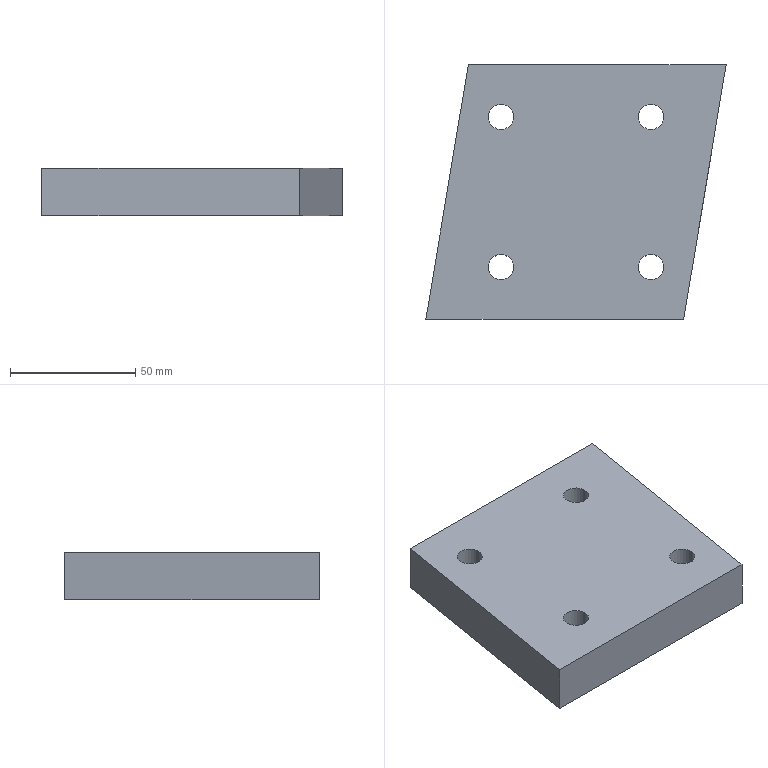Part | SolidWorks | features BaseBody 1 | 1 solid | 14 faces | box 120.015 x 101.6 x 19 mm | volume 192760 mm3 | cylinder 8 | plane 6 | commonest cylinder face diameters 10.106 x8
STEP:
#1=CARTESIAN_POINT('',(16.587,73.951,0.));
#2=VERTEX_POINT('',#1);
#3=CARTESIAN_POINT('',(6.481,73.951,0.));
#4=VERTEX_POINT('',#3);
#5=CARTESIAN_POINT('',(11.534,73.951,0.));
#6=DIRECTION('',(0.,0.,-1.));
#7=DIRECTION('',(1.,0.,0.));
#8=AXIS2_PLACEMENT_3D('',#5,#6,#7);
#9=CIRCLE('',#8,5.053);
#10=EDGE_CURVE('',#2,#4,#9,.T.);
#11=ORIENTED_EDGE('',*,*,#10,.T.);
#12=CARTESIAN_POINT('',(6.481,73.951,19.));
#13=VERTEX_POINT('',#12);
#14=CARTESIAN_POINT('',(6.481,73.951,-272.723));
#15=DIRECTION('',(0.,0.,1.));
#16=VECTOR('',#15,1000.);
#17=LINE('',#14,#16);
#18=EDGE_CURVE('',#4,#13,#17,.T.);
#19=ORIENTED_EDGE('',*,*,#18,.T.);
#20=CARTESIAN_POINT('',(16.587,73.951,19.));
#21=VERTEX_POINT('',#20);
#22=CARTESIAN_POINT('',(11.534,73.951,19.));
#23=DIRECTION('',(0.,0.,-1.));
#24=DIRECTION('',(1.,0.,0.));
#25=AXIS2_PLACEMENT_3D('',#22,#23,#24);
#26=CIRCLE('',#25,5.053);
#27=EDGE_CURVE('',#21,#13,#26,.T.);
#28=ORIENTED_EDGE('',*,*,#27,.F.);
#29=CARTESIAN_POINT('',(16.587,73.951,-272.723));
#30=DIRECTION('',(0.,0.,1.));
#31=VECTOR('',#30,1000.);
#32=LINE('',#29,#31);
#33=EDGE_CURVE('',#2,#21,#32,.T.);
#34=ORIENTED_EDGE('',*,*,#33,.F.);
#35=EDGE_LOOP('',(#11,#19,#28,#34));
#36=FACE_OUTER_BOUND('',#35,.T.);
#37=CARTESIAN_POINT('',(11.534,73.951,-272.723));
#38=DIRECTION('',(0.,0.,1.));
#39=DIRECTION('',(1.,0.,0.));
#40=AXIS2_PLACEMENT_3D('',#37,#38,#39);
#41=CYLINDRICAL_SURFACE('',#40,5.053);
#42=ADVANCED_FACE('',(#36),#41,.F.);
#43=CARTESIAN_POINT('',(76.587,73.951,0.));
#44=VERTEX_POINT('',#43);
#45=CARTESIAN_POINT('',(66.481,73.951,0.));
#46=VERTEX_POINT('',#45);
#47=CARTESIAN_POINT('',(71.534,73.951,0.));
#48=DIRECTION('',(0.,0.,-1.));
#49=DIRECTION('',(1.,0.,0.));
#50=AXIS2_PLACEMENT_3D('',#47,#48,#49);
#51=CIRCLE('',#50,5.053);
#52=EDGE_CURVE('',#44,#46,#51,.T.);
#53=ORIENTED_EDGE('',*,*,#52,.T.);
#54=CARTESIAN_POINT('',(66.481,73.951,19.));
#55=VERTEX_POINT('',#54);
#56=CARTESIAN_POINT('',(66.481,73.951,-272.723));
#57=DIRECTION('',(0.,0.,1.));
#58=VECTOR('',#57,1000.);
#59=LINE('',#56,#58);
#60=EDGE_CURVE('',#46,#55,#59,.T.);
#61=ORIENTED_EDGE('',*,*,#60,.T.);
#62=CARTESIAN_POINT('',(76.587,73.951,19.));
#63=VERTEX_POINT('',#62);
#64=CARTESIAN_POINT('',(71.534,73.951,19.));
#65=DIRECTION('',(0.,0.,-1.));
#66=DIRECTION('',(1.,0.,0.));
#67=AXIS2_PLACEMENT_3D('',#64,#65,#66);
#68=CIRCLE('',#67,5.053);
#69=EDGE_CURVE('',#63,#55,#68,.T.);
#70=ORIENTED_EDGE('',*,*,#69,.F.);
#71=CARTESIAN_POINT('',(76.587,73.951,-272.723));
#72=DIRECTION('',(0.,0.,1.));
#73=VECTOR('',#72,1000.);
#74=LINE('',#71,#73);
#75=EDGE_CURVE('',#44,#63,#74,.T.);
#76=ORIENTED_EDGE('',*,*,#75,.F.);
#77=EDGE_LOOP('',(#53,#61,#70,#76));
#78=FACE_OUTER_BOUND('',#77,.T.);
#79=CARTESIAN_POINT('',(71.534,73.951,-272.723));
#80=DIRECTION('',(0.,0.,1.));
#81=DIRECTION('',(1.,0.,0.));
#82=AXIS2_PLACEMENT_3D('',#79,#80,#81);
#83=CYLINDRICAL_SURFACE('',#82,5.053);
#84=ADVANCED_FACE('',(#78),#83,.F.);
#85=CARTESIAN_POINT('',(76.587,13.951,0.));
#86=VERTEX_POINT('',#85);
#87=CARTESIAN_POINT('',(66.481,13.951,0.));
#88=VERTEX_POINT('',#87);
#89=CARTESIAN_POINT('',(71.534,13.951,0.));
#90=DIRECTION('',(0.,0.,-1.));
#91=DIRECTION('',(1.,0.,0.));
#92=AXIS2_PLACEMENT_3D('',#89,#90,#91);
#93=CIRCLE('',#92,5.053);
#94=EDGE_CURVE('',#86,#88,#93,.T.);
#95=ORIENTED_EDGE('',*,*,#94,.T.);
#96=CARTESIAN_POINT('',(66.481,13.951,19.));
#97=VERTEX_POINT('',#96);
#98=CARTESIAN_POINT('',(66.481,13.951,-272.723));
#99=DIRECTION('',(0.,0.,1.));
#100=VECTOR('',#99,1000.);
#101=LINE('',#98,#100);
#102=EDGE_CURVE('',#88,#97,#101,.T.);
#103=ORIENTED_EDGE('',*,*,#102,.T.);
#104=CARTESIAN_POINT('',(76.587,13.951,19.));
#105=VERTEX_POINT('',#104);
#106=CARTESIAN_POINT('',(71.534,13.951,19.));
#107=DIRECTION('',(0.,0.,-1.));
#108=DIRECTION('',(1.,0.,0.));
#109=AXIS2_PLACEMENT_3D('',#106,#107,#108);
#110=CIRCLE('',#109,5.053);
#111=EDGE_CURVE('',#105,#97,#110,.T.);
#112=ORIENTED_EDGE('',*,*,#111,.F.);
#113=CARTESIAN_POINT('',(76.587,13.951,-272.723));
#114=DIRECTION('',(0.,0.,1.));
#115=VECTOR('',#114,1000.);
#116=LINE('',#113,#115);
#117=EDGE_CURVE('',#86,#105,#116,.T.);
#118=ORIENTED_EDGE('',*,*,#117,.F.);
#119=EDGE_LOOP('',(#95,#103,#112,#118));
#120=FACE_OUTER_BOUND('',#119,.T.);
#121=CARTESIAN_POINT('',(71.534,13.951,-272.723));
#122=DIRECTION('',(0.,0.,1.));
#123=DIRECTION('',(1.,0.,0.));
#124=AXIS2_PLACEMENT_3D('',#121,#122,#123);
#125=CYLINDRICAL_SURFACE('',#124,5.053);
#126=ADVANCED_FACE('',(#120),#125,.F.);
#127=CARTESIAN_POINT('',(16.587,13.951,0.));
#128=VERTEX_POINT('',#127);
#129=CARTESIAN_POINT('',(6.481,13.951,0.));
#130=VERTEX_POINT('',#129);
#131=CARTESIAN_POINT('',(11.534,13.951,0.));
#132=DIRECTION('',(0.,0.,-1.));
#133=DIRECTION('',(1.,0.,0.));
#134=AXIS2_PLACEMENT_3D('',#131,#132,#133);
#135=CIRCLE('',#134,5.053);
#136=EDGE_CURVE('',#128,#130,#135,.T.);
#137=ORIENTED_EDGE('',*,*,#136,.T.);
#138=CARTESIAN_POINT('',(6.481,13.951,19.));
#139=VERTEX_POINT('',#138);
#140=CARTESIAN_POINT('',(6.481,13.951,-272.723));
#141=DIRECTION('',(0.,0.,1.));
#142=VECTOR('',#141,1000.);
#143=LINE('',#140,#142);
#144=EDGE_CURVE('',#130,#139,#143,.T.);
#145=ORIENTED_EDGE('',*,*,#144,.T.);
#146=CARTESIAN_POINT('',(16.587,13.951,19.));
#147=VERTEX_POINT('',#146);
#148=CARTESIAN_POINT('',(11.534,13.951,19.));
#149=DIRECTION('',(0.,0.,-1.));
#150=DIRECTION('',(1.,0.,0.));
#151=AXIS2_PLACEMENT_3D('',#148,#149,#150);
#152=CIRCLE('',#151,5.053);
#153=EDGE_CURVE('',#147,#139,#152,.T.);
#154=ORIENTED_EDGE('',*,*,#153,.F.);
#155=CARTESIAN_POINT('',(16.587,13.951,-272.723));
#156=DIRECTION('',(0.,0.,1.));
#157=VECTOR('',#156,1000.);
#158=LINE('',#155,#157);
#159=EDGE_CURVE('',#128,#147,#158,.T.);
#160=ORIENTED_EDGE('',*,*,#159,.F.);
#161=EDGE_LOOP('',(#137,#145,#154,#160));
#162=FACE_OUTER_BOUND('',#161,.T.);
#163=CARTESIAN_POINT('',(11.534,13.951,-272.723));
#164=DIRECTION('',(0.,0.,1.));
#165=DIRECTION('',(1.,0.,0.));
#166=AXIS2_PLACEMENT_3D('',#163,#164,#165);
#167=CYLINDRICAL_SURFACE('',#166,5.053);
#168=ADVANCED_FACE('',(#162),#167,.F.);
#169=ORIENTED_EDGE('',*,*,#10,.F.);
#170=CARTESIAN_POINT('',(11.534,73.951,0.));
#171=DIRECTION('',(0.,0.,-1.));
#172=DIRECTION('',(1.,0.,0.));
#173=AXIS2_PLACEMENT_3D('',#170,#171,#172);
#174=CIRCLE('',#173,5.053);
#175=EDGE_CURVE('',#4,#2,#174,.T.);
#176=ORIENTED_EDGE('',*,*,#175,.F.);
#177=EDGE_LOOP('',(#169,#176));
#178=FACE_BOUND('',#177,.T.);
#179=ORIENTED_EDGE('',*,*,#52,.F.);
#180=CARTESIAN_POINT('',(71.534,73.951,0.));
#181=DIRECTION('',(0.,0.,-1.));
#182=DIRECTION('',(1.,0.,0.));
#183=AXIS2_PLACEMENT_3D('',#180,#181,#182);
#184=CIRCLE('',#183,5.053);
#185=EDGE_CURVE('',#46,#44,#184,.T.);
#186=ORIENTED_EDGE('',*,*,#185,.F.);
#187=EDGE_LOOP('',(#179,#186));
#188=FACE_BOUND('',#187,.T.);
#189=ORIENTED_EDGE('',*,*,#94,.F.);
#190=CARTESIAN_POINT('',(71.534,13.951,0.));
#191=DIRECTION('',(0.,0.,-1.));
#192=DIRECTION('',(1.,0.,0.));
#193=AXIS2_PLACEMENT_3D('',#190,#191,#192);
#194=CIRCLE('',#193,5.053);
#195=EDGE_CURVE('',#88,#86,#194,.T.);
#196=ORIENTED_EDGE('',*,*,#195,.F.);
#197=EDGE_LOOP('',(#189,#196));
#198=FACE_BOUND('',#197,.T.);
#199=ORIENTED_EDGE('',*,*,#136,.F.);
#200=CARTESIAN_POINT('',(11.534,13.951,0.));
#201=DIRECTION('',(0.,0.,-1.));
#202=DIRECTION('',(1.,0.,0.));
#203=AXIS2_PLACEMENT_3D('',#200,#201,#202);
#204=CIRCLE('',#203,5.053);
#205=EDGE_CURVE('',#130,#128,#204,.T.);
#206=ORIENTED_EDGE('',*,*,#205,.F.);
#207=EDGE_LOOP('',(#199,#206));
#208=FACE_BOUND('',#207,.T.);
#209=CARTESIAN_POINT('',(101.541,94.751,0.));
#210=VERTEX_POINT('',#209);
#211=CARTESIAN_POINT('',(-1.472,94.751,0.));
#212=VERTEX_POINT('',#211);
#213=CARTESIAN_POINT('',(41.534,94.751,0.));
#214=DIRECTION('',(-1.,0.,0.));
#215=VECTOR('',#214,1000.);
#216=LINE('',#213,#215);
#217=EDGE_CURVE('',#210,#212,#216,.T.);
#218=ORIENTED_EDGE('',*,*,#217,.F.);
#219=CARTESIAN_POINT('',(84.539,-6.849,0.));
#220=VERTEX_POINT('',#219);
#221=CARTESIAN_POINT('',(84.539,-6.849,0.));
#222=DIRECTION('',(0.165,0.9863,0.));
#223=VECTOR('',#222,1000.);
#224=LINE('',#221,#223);
#225=EDGE_CURVE('',#220,#210,#224,.T.);
#226=ORIENTED_EDGE('',*,*,#225,.F.);
#227=CARTESIAN_POINT('',(-18.474,-6.849,0.));
#228=VERTEX_POINT('',#227);
#229=CARTESIAN_POINT('',(41.534,-6.849,0.));
#230=DIRECTION('',(1.,0.,0.));
#231=VECTOR('',#230,1000.);
#232=LINE('',#229,#231);
#233=EDGE_CURVE('',#228,#220,#232,.T.);
#234=ORIENTED_EDGE('',*,*,#233,.F.);
#235=CARTESIAN_POINT('',(-1.472,94.751,0.));
#236=DIRECTION('',(-0.165,-0.9863,0.));
#237=VECTOR('',#236,1000.);
#238=LINE('',#235,#237);
#239=EDGE_CURVE('',#212,#228,#238,.T.);
#240=ORIENTED_EDGE('',*,*,#239,.F.);
#241=EDGE_LOOP('',(#218,#226,#234,#240));
#242=FACE_OUTER_BOUND('',#241,.T.);
#243=CARTESIAN_POINT('',(41.534,43.951,0.));
#244=DIRECTION('',(0.,0.,1.));
#245=DIRECTION('',(1.,0.,0.));
#246=AXIS2_PLACEMENT_3D('',#243,#244,#245);
#247=PLANE('',#246);
#248=ADVANCED_FACE('',(#178,#188,#198,#208,#242),#247,.F.);
#249=ORIENTED_EDGE('',*,*,#18,.F.);
#250=ORIENTED_EDGE('',*,*,#175,.T.);
#251=ORIENTED_EDGE('',*,*,#33,.T.);
#252=CARTESIAN_POINT('',(11.534,73.951,19.));
#253=DIRECTION('',(0.,0.,-1.));
#254=DIRECTION('',(1.,0.,0.));
#255=AXIS2_PLACEMENT_3D('',#252,#253,#254);
#256=CIRCLE('',#255,5.053);
#257=EDGE_CURVE('',#13,#21,#256,.T.);
#258=ORIENTED_EDGE('',*,*,#257,.F.);
#259=EDGE_LOOP('',(#249,#250,#251,#258));
#260=FACE_OUTER_BOUND('',#259,.T.);
#261=CARTESIAN_POINT('',(11.534,73.951,-272.723));
#262=DIRECTION('',(0.,0.,1.));
#263=DIRECTION('',(1.,0.,0.));
#264=AXIS2_PLACEMENT_3D('',#261,#262,#263);
#265=CYLINDRICAL_SURFACE('',#264,5.053);
#266=ADVANCED_FACE('',(#260),#265,.F.);
#267=ORIENTED_EDGE('',*,*,#60,.F.);
#268=ORIENTED_EDGE('',*,*,#185,.T.);
#269=ORIENTED_EDGE('',*,*,#75,.T.);
#270=CARTESIAN_POINT('',(71.534,73.951,19.));
#271=DIRECTION('',(0.,0.,-1.));
#272=DIRECTION('',(1.,0.,0.));
#273=AXIS2_PLACEMENT_3D('',#270,#271,#272);
#274=CIRCLE('',#273,5.053);
#275=EDGE_CURVE('',#55,#63,#274,.T.);
#276=ORIENTED_EDGE('',*,*,#275,.F.);
#277=EDGE_LOOP('',(#267,#268,#269,#276));
#278=FACE_OUTER_BOUND('',#277,.T.);
#279=CARTESIAN_POINT('',(71.534,73.951,-272.723));
#280=DIRECTION('',(0.,0.,1.));
#281=DIRECTION('',(1.,0.,0.));
#282=AXIS2_PLACEMENT_3D('',#279,#280,#281);
#283=CYLINDRICAL_SURFACE('',#282,5.053);
#284=ADVANCED_FACE('',(#278),#283,.F.);
#285=ORIENTED_EDGE('',*,*,#102,.F.);
#286=ORIENTED_EDGE('',*,*,#195,.T.);
#287=ORIENTED_EDGE('',*,*,#117,.T.);
#288=CARTESIAN_POINT('',(71.534,13.951,19.));
#289=DIRECTION('',(0.,0.,-1.));
#290=DIRECTION('',(1.,0.,0.));
#291=AXIS2_PLACEMENT_3D('',#288,#289,#290);
#292=CIRCLE('',#291,5.053);
#293=EDGE_CURVE('',#97,#105,#292,.T.);
#294=ORIENTED_EDGE('',*,*,#293,.F.);
#295=EDGE_LOOP('',(#285,#286,#287,#294));
#296=FACE_OUTER_BOUND('',#295,.T.);
#297=CARTESIAN_POINT('',(71.534,13.951,-272.723));
#298=DIRECTION('',(0.,0.,1.));
#299=DIRECTION('',(1.,0.,0.));
#300=AXIS2_PLACEMENT_3D('',#297,#298,#299);
#301=CYLINDRICAL_SURFACE('',#300,5.053);
#302=ADVANCED_FACE('',(#296),#301,.F.);
#303=ORIENTED_EDGE('',*,*,#144,.F.);
#304=ORIENTED_EDGE('',*,*,#205,.T.);
#305=ORIENTED_EDGE('',*,*,#159,.T.);
#306=CARTESIAN_POINT('',(11.534,13.951,19.));
#307=DIRECTION('',(0.,0.,-1.));
#308=DIRECTION('',(1.,0.,0.));
#309=AXIS2_PLACEMENT_3D('',#306,#307,#308);
#310=CIRCLE('',#309,5.053);
#311=EDGE_CURVE('',#139,#147,#310,.T.);
#312=ORIENTED_EDGE('',*,*,#311,.F.);
#313=EDGE_LOOP('',(#303,#304,#305,#312));
#314=FACE_OUTER_BOUND('',#313,.T.);
#315=CARTESIAN_POINT('',(11.534,13.951,-272.723));
#316=DIRECTION('',(0.,0.,1.));
#317=DIRECTION('',(1.,0.,0.));
#318=AXIS2_PLACEMENT_3D('',#315,#316,#317);
#319=CYLINDRICAL_SURFACE('',#318,5.053);
#320=ADVANCED_FACE('',(#314),#319,.F.);
#321=ORIENTED_EDGE('',*,*,#239,.T.);
#322=CARTESIAN_POINT('',(-18.474,-6.849,19.));
#323=VERTEX_POINT('',#322);
#324=CARTESIAN_POINT('',(-18.474,-6.849,0.));
#325=DIRECTION('',(0.,0.,1.));
#326=VECTOR('',#325,1000.);
#327=LINE('',#324,#326);
#328=EDGE_CURVE('',#228,#323,#327,.T.);
#329=ORIENTED_EDGE('',*,*,#328,.T.);
#330=CARTESIAN_POINT('',(-1.472,94.751,19.));
#331=VERTEX_POINT('',#330);
#332=CARTESIAN_POINT('',(-18.474,-6.849,19.));
#333=DIRECTION('',(0.165,0.9863,0.));
#334=VECTOR('',#333,1000.);
#335=LINE('',#332,#334);
#336=EDGE_CURVE('',#323,#331,#335,.T.);
#337=ORIENTED_EDGE('',*,*,#336,.T.);
#338=CARTESIAN_POINT('',(-1.472,94.751,0.));
#339=DIRECTION('',(0.,0.,-1.));
#340=VECTOR('',#339,1000.);
#341=LINE('',#338,#340);
#342=EDGE_CURVE('',#331,#212,#341,.T.);
#343=ORIENTED_EDGE('',*,*,#342,.T.);
#344=EDGE_LOOP('',(#321,#329,#337,#343));
#345=FACE_OUTER_BOUND('',#344,.T.);
#346=CARTESIAN_POINT('',(-18.474,-6.849,0.));
#347=DIRECTION('',(-0.9863,0.165,0.));
#348=DIRECTION('',(-0.165,-0.9863,0.));
#349=AXIS2_PLACEMENT_3D('',#346,#347,#348);
#350=PLANE('',#349);
#351=ADVANCED_FACE('',(#345),#350,.T.);
#352=ORIENTED_EDGE('',*,*,#217,.T.);
#353=ORIENTED_EDGE('',*,*,#342,.F.);
#354=CARTESIAN_POINT('',(101.541,94.751,19.));
#355=VERTEX_POINT('',#354);
#356=CARTESIAN_POINT('',(-1.472,94.751,19.));
#357=DIRECTION('',(1.,0.,0.));
#358=VECTOR('',#357,1000.);
#359=LINE('',#356,#358);
#360=EDGE_CURVE('',#331,#355,#359,.T.);
#361=ORIENTED_EDGE('',*,*,#360,.T.);
#362=CARTESIAN_POINT('',(101.541,94.751,0.));
#363=DIRECTION('',(0.,0.,-1.));
#364=VECTOR('',#363,1000.);
#365=LINE('',#362,#364);
#366=EDGE_CURVE('',#355,#210,#365,.T.);
#367=ORIENTED_EDGE('',*,*,#366,.T.);
#368=EDGE_LOOP('',(#352,#353,#361,#367));
#369=FACE_OUTER_BOUND('',#368,.T.);
#370=CARTESIAN_POINT('',(-1.472,94.751,0.));
#371=DIRECTION('',(0.,1.,0.));
#372=DIRECTION('',(0.,0.,1.));
#373=AXIS2_PLACEMENT_3D('',#370,#371,#372);
#374=PLANE('',#373);
#375=ADVANCED_FACE('',(#369),#374,.T.);
#376=ORIENTED_EDGE('',*,*,#225,.T.);
#377=ORIENTED_EDGE('',*,*,#366,.F.);
#378=CARTESIAN_POINT('',(84.539,-6.849,19.));
#379=VERTEX_POINT('',#378);
#380=CARTESIAN_POINT('',(101.541,94.751,19.));
#381=DIRECTION('',(-0.165,-0.9863,0.));
#382=VECTOR('',#381,1000.);
#383=LINE('',#380,#382);
#384=EDGE_CURVE('',#355,#379,#383,.T.);
#385=ORIENTED_EDGE('',*,*,#384,.T.);
#386=CARTESIAN_POINT('',(84.539,-6.849,0.));
#387=DIRECTION('',(0.,0.,-1.));
#388=VECTOR('',#387,1000.);
#389=LINE('',#386,#388);
#390=EDGE_CURVE('',#379,#220,#389,.T.);
#391=ORIENTED_EDGE('',*,*,#390,.T.);
#392=EDGE_LOOP('',(#376,#377,#385,#391));
#393=FACE_OUTER_BOUND('',#392,.T.);
#394=CARTESIAN_POINT('',(101.541,94.751,0.));
#395=DIRECTION('',(0.9863,-0.165,0.));
#396=DIRECTION('',(0.165,0.9863,0.));
#397=AXIS2_PLACEMENT_3D('',#394,#395,#396);
#398=PLANE('',#397);
#399=ADVANCED_FACE('',(#393),#398,.T.);
#400=ORIENTED_EDGE('',*,*,#233,.T.);
#401=ORIENTED_EDGE('',*,*,#390,.F.);
#402=CARTESIAN_POINT('',(84.539,-6.849,19.));
#403=DIRECTION('',(-1.,0.,0.));
#404=VECTOR('',#403,1000.);
#405=LINE('',#402,#404);
#406=EDGE_CURVE('',#379,#323,#405,.T.);
#407=ORIENTED_EDGE('',*,*,#406,.T.);
#408=ORIENTED_EDGE('',*,*,#328,.F.);
#409=EDGE_LOOP('',(#400,#401,#407,#408));
#410=FACE_OUTER_BOUND('',#409,.T.);
#411=CARTESIAN_POINT('',(84.539,-6.849,0.));
#412=DIRECTION('',(0.,-1.,0.));
#413=DIRECTION('',(0.,0.,-1.));
#414=AXIS2_PLACEMENT_3D('',#411,#412,#413);
#415=PLANE('',#414);
#416=ADVANCED_FACE('',(#410),#415,.T.);
#417=ORIENTED_EDGE('',*,*,#27,.T.);
#418=ORIENTED_EDGE('',*,*,#257,.T.);
#419=EDGE_LOOP('',(#417,#418));
#420=FACE_BOUND('',#419,.T.);
#421=ORIENTED_EDGE('',*,*,#69,.T.);
#422=ORIENTED_EDGE('',*,*,#275,.T.);
#423=EDGE_LOOP('',(#421,#422));
#424=FACE_BOUND('',#423,.T.);
#425=ORIENTED_EDGE('',*,*,#111,.T.);
#426=ORIENTED_EDGE('',*,*,#293,.T.);
#427=EDGE_LOOP('',(#425,#426));
#428=FACE_BOUND('',#427,.T.);
#429=ORIENTED_EDGE('',*,*,#153,.T.);
#430=ORIENTED_EDGE('',*,*,#311,.T.);
#431=EDGE_LOOP('',(#429,#430));
#432=FACE_BOUND('',#431,.T.);
#433=ORIENTED_EDGE('',*,*,#406,.F.);
#434=ORIENTED_EDGE('',*,*,#384,.F.);
#435=ORIENTED_EDGE('',*,*,#360,.F.);
#436=ORIENTED_EDGE('',*,*,#336,.F.);
#437=EDGE_LOOP('',(#433,#434,#435,#436));
#438=FACE_OUTER_BOUND('',#437,.T.);
#439=CARTESIAN_POINT('',(41.534,43.951,19.));
#440=DIRECTION('',(0.,0.,1.));
#441=DIRECTION('',(1.,0.,0.));
#442=AXIS2_PLACEMENT_3D('',#439,#440,#441);
#443=PLANE('',#442);
#444=ADVANCED_FACE('',(#420,#424,#428,#432,#438),#443,.T.);
#445=CLOSED_SHELL('',(#42,#84,#126,#168,#248,#266,#284,#302,#320,#351,#375,#399,#416,#444));
#446=MANIFOLD_SOLID_BREP('',#445);
#447=CARTESIAN_POINT('',(0.,0.,0.));
#448=DIRECTION('',(0.,0.,1.));
#449=DIRECTION('',(1.,0.,0.));
#450=AXIS2_PLACEMENT_3D('',#447,#448,#449);
#451=(LENGTH_UNIT()NAMED_UNIT(*)SI_UNIT(.MILLI.,.METRE.));
#452=UNCERTAINTY_MEASURE_WITH_UNIT(LENGTH_MEASURE(0.00001),#451,'','');
#453=(NAMED_UNIT(*)PLANE_ANGLE_UNIT()SI_UNIT($,.RADIAN.));
#454=(NAMED_UNIT(*)SI_UNIT($,.STERADIAN.)SOLID_ANGLE_UNIT());
#455=(GEOMETRIC_REPRESENTATION_CONTEXT(3)GLOBAL_UNCERTAINTY_ASSIGNED_CONTEXT((#452))GLOBAL_UNIT_ASSIGNED_CONTEXT((#451,#453,#454))REPRESENTATION_CONTEXT('',''));
#456=ADVANCED_BREP_SHAPE_REPRESENTATION('',(#446,#450),#455);